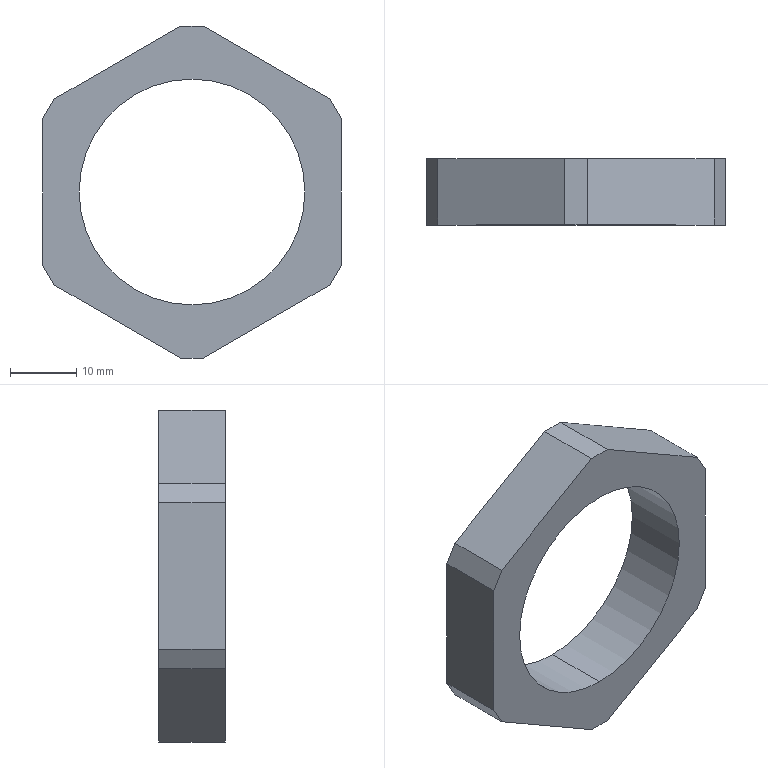Part | SolidWorks | features CirPattern 1, Extrusion 1, HoleWzd 1, ICE 1 | 1 solid | 16 faces | box 45 x 10 x 50 mm | volume 8358 mm3 | plane 14 | cylinder 2 | commonest cylinder face diameters 34 x2
STEP:
#1=CARTESIAN_POINT('',(0.,0.,-17.));
#2=VERTEX_POINT('',#1);
#3=CARTESIAN_POINT('',(0.,0.,17.));
#4=VERTEX_POINT('',#3);
#5=CARTESIAN_POINT('',(0.,0.,0.));
#6=DIRECTION('',(0.,1.,0.));
#7=DIRECTION('',(0.,0.,1.));
#8=AXIS2_PLACEMENT_3D('',#5,#6,#7);
#9=CIRCLE('',#8,17.);
#10=EDGE_CURVE('',#2,#4,#9,.T.);
#11=ORIENTED_EDGE('',*,*,#10,.F.);
#12=CARTESIAN_POINT('',(0.,10.,-17.));
#13=VERTEX_POINT('',#12);
#14=CARTESIAN_POINT('',(0.,10.,-17.));
#15=DIRECTION('',(0.,1.,0.));
#16=VECTOR('',#15,1000.);
#17=LINE('',#14,#16);
#18=EDGE_CURVE('',#2,#13,#17,.T.);
#19=ORIENTED_EDGE('',*,*,#18,.T.);
#20=CARTESIAN_POINT('',(0.,10.,17.));
#21=VERTEX_POINT('',#20);
#22=CARTESIAN_POINT('',(0.,10.,0.));
#23=DIRECTION('',(0.,1.,0.));
#24=DIRECTION('',(0.,0.,1.));
#25=AXIS2_PLACEMENT_3D('',#22,#23,#24);
#26=CIRCLE('',#25,17.);
#27=EDGE_CURVE('',#13,#21,#26,.T.);
#28=ORIENTED_EDGE('',*,*,#27,.T.);
#29=CARTESIAN_POINT('',(0.,10.,17.));
#30=DIRECTION('',(0.,1.,0.));
#31=VECTOR('',#30,1000.);
#32=LINE('',#29,#31);
#33=EDGE_CURVE('',#4,#21,#32,.T.);
#34=ORIENTED_EDGE('',*,*,#33,.F.);
#35=EDGE_LOOP('',(#11,#19,#28,#34));
#36=FACE_OUTER_BOUND('',#35,.T.);
#37=CARTESIAN_POINT('',(0.,10.,0.));
#38=DIRECTION('',(0.,1.,0.));
#39=DIRECTION('',(0.,0.,1.));
#40=AXIS2_PLACEMENT_3D('',#37,#38,#39);
#41=CYLINDRICAL_SURFACE('',#40,17.);
#42=ADVANCED_FACE('',(#36),#41,.F.);
#43=CARTESIAN_POINT('',(1.699,0.,25.));
#44=VERTEX_POINT('',#43);
#45=CARTESIAN_POINT('',(20.801,0.,13.971));
#46=VERTEX_POINT('',#45);
#47=CARTESIAN_POINT('',(0.,0.,25.981));
#48=DIRECTION('',(0.866,0.,-0.5));
#49=VECTOR('',#48,1000.);
#50=LINE('',#47,#49);
#51=EDGE_CURVE('',#44,#46,#50,.T.);
#52=ORIENTED_EDGE('',*,*,#51,.T.);
#53=CARTESIAN_POINT('',(20.801,10.,13.971));
#54=VERTEX_POINT('',#53);
#55=CARTESIAN_POINT('',(20.801,10.,13.971));
#56=DIRECTION('',(0.,1.,0.));
#57=VECTOR('',#56,1000.);
#58=LINE('',#55,#57);
#59=EDGE_CURVE('',#46,#54,#58,.T.);
#60=ORIENTED_EDGE('',*,*,#59,.T.);
#61=CARTESIAN_POINT('',(1.699,10.,25.));
#62=VERTEX_POINT('',#61);
#63=CARTESIAN_POINT('',(0.,10.,25.981));
#64=DIRECTION('',(0.866,0.,-0.5));
#65=VECTOR('',#64,1000.);
#66=LINE('',#63,#65);
#67=EDGE_CURVE('',#62,#54,#66,.T.);
#68=ORIENTED_EDGE('',*,*,#67,.F.);
#69=CARTESIAN_POINT('',(1.699,10.,25.));
#70=DIRECTION('',(0.,-1.,0.));
#71=VECTOR('',#70,1000.);
#72=LINE('',#69,#71);
#73=EDGE_CURVE('',#62,#44,#72,.T.);
#74=ORIENTED_EDGE('',*,*,#73,.T.);
#75=EDGE_LOOP('',(#52,#60,#68,#74));
#76=FACE_OUTER_BOUND('',#75,.T.);
#77=CARTESIAN_POINT('',(0.,10.,25.981));
#78=DIRECTION('',(-0.5,0.,-0.866));
#79=DIRECTION('',(-0.866,0.,0.5));
#80=AXIS2_PLACEMENT_3D('',#77,#78,#79);
#81=PLANE('',#80);
#82=ADVANCED_FACE('',(#76),#81,.F.);
#83=CARTESIAN_POINT('',(22.5,0.,11.029));
#84=VERTEX_POINT('',#83);
#85=CARTESIAN_POINT('',(22.5,0.,-11.029));
#86=VERTEX_POINT('',#85);
#87=CARTESIAN_POINT('',(22.5,0.,12.99));
#88=DIRECTION('',(0.,0.,-1.));
#89=VECTOR('',#88,1000.);
#90=LINE('',#87,#89);
#91=EDGE_CURVE('',#84,#86,#90,.T.);
#92=ORIENTED_EDGE('',*,*,#91,.T.);
#93=CARTESIAN_POINT('',(22.5,10.,-11.029));
#94=VERTEX_POINT('',#93);
#95=CARTESIAN_POINT('',(22.5,10.,-11.029));
#96=DIRECTION('',(0.,1.,0.));
#97=VECTOR('',#96,1000.);
#98=LINE('',#95,#97);
#99=EDGE_CURVE('',#86,#94,#98,.T.);
#100=ORIENTED_EDGE('',*,*,#99,.T.);
#101=CARTESIAN_POINT('',(22.5,10.,11.029));
#102=VERTEX_POINT('',#101);
#103=CARTESIAN_POINT('',(22.5,10.,12.99));
#104=DIRECTION('',(0.,0.,-1.));
#105=VECTOR('',#104,1000.);
#106=LINE('',#103,#105);
#107=EDGE_CURVE('',#102,#94,#106,.T.);
#108=ORIENTED_EDGE('',*,*,#107,.F.);
#109=CARTESIAN_POINT('',(22.5,10.,11.029));
#110=DIRECTION('',(0.,-1.,0.));
#111=VECTOR('',#110,1000.);
#112=LINE('',#109,#111);
#113=EDGE_CURVE('',#102,#84,#112,.T.);
#114=ORIENTED_EDGE('',*,*,#113,.T.);
#115=EDGE_LOOP('',(#92,#100,#108,#114));
#116=FACE_OUTER_BOUND('',#115,.T.);
#117=CARTESIAN_POINT('',(22.5,10.,12.99));
#118=DIRECTION('',(-1.,0.,0.));
#119=DIRECTION('',(0.,0.,1.));
#120=AXIS2_PLACEMENT_3D('',#117,#118,#119);
#121=PLANE('',#120);
#122=ADVANCED_FACE('',(#116),#121,.F.);
#123=CARTESIAN_POINT('',(20.801,10.,-13.971));
#124=VERTEX_POINT('',#123);
#125=CARTESIAN_POINT('',(1.699,10.,-25.));
#126=VERTEX_POINT('',#125);
#127=CARTESIAN_POINT('',(22.5,10.,-12.99));
#128=DIRECTION('',(-0.866,0.,-0.5));
#129=VECTOR('',#128,1000.);
#130=LINE('',#127,#129);
#131=EDGE_CURVE('',#124,#126,#130,.T.);
#132=ORIENTED_EDGE('',*,*,#131,.F.);
#133=CARTESIAN_POINT('',(20.801,0.,-13.971));
#134=VERTEX_POINT('',#133);
#135=CARTESIAN_POINT('',(20.801,10.,-13.971));
#136=DIRECTION('',(0.,-1.,0.));
#137=VECTOR('',#136,1000.);
#138=LINE('',#135,#137);
#139=EDGE_CURVE('',#124,#134,#138,.T.);
#140=ORIENTED_EDGE('',*,*,#139,.T.);
#141=CARTESIAN_POINT('',(1.699,0.,-25.));
#142=VERTEX_POINT('',#141);
#143=CARTESIAN_POINT('',(22.5,0.,-12.99));
#144=DIRECTION('',(-0.866,0.,-0.5));
#145=VECTOR('',#144,1000.);
#146=LINE('',#143,#145);
#147=EDGE_CURVE('',#134,#142,#146,.T.);
#148=ORIENTED_EDGE('',*,*,#147,.T.);
#149=CARTESIAN_POINT('',(1.699,10.,-25.));
#150=DIRECTION('',(0.,1.,0.));
#151=VECTOR('',#150,1000.);
#152=LINE('',#149,#151);
#153=EDGE_CURVE('',#142,#126,#152,.T.);
#154=ORIENTED_EDGE('',*,*,#153,.T.);
#155=EDGE_LOOP('',(#132,#140,#148,#154));
#156=FACE_OUTER_BOUND('',#155,.T.);
#157=CARTESIAN_POINT('',(22.5,10.,-12.99));
#158=DIRECTION('',(-0.5,0.,0.866));
#159=DIRECTION('',(0.866,0.,0.5));
#160=AXIS2_PLACEMENT_3D('',#157,#158,#159);
#161=PLANE('',#160);
#162=ADVANCED_FACE('',(#156),#161,.F.);
#163=CARTESIAN_POINT('',(-1.699,0.,-25.));
#164=VERTEX_POINT('',#163);
#165=CARTESIAN_POINT('',(-20.801,0.,-13.971));
#166=VERTEX_POINT('',#165);
#167=CARTESIAN_POINT('',(0.,0.,-25.981));
#168=DIRECTION('',(-0.866,0.,0.5));
#169=VECTOR('',#168,1000.);
#170=LINE('',#167,#169);
#171=EDGE_CURVE('',#164,#166,#170,.T.);
#172=ORIENTED_EDGE('',*,*,#171,.T.);
#173=CARTESIAN_POINT('',(-20.801,10.,-13.971));
#174=VERTEX_POINT('',#173);
#175=CARTESIAN_POINT('',(-20.801,10.,-13.971));
#176=DIRECTION('',(0.,1.,0.));
#177=VECTOR('',#176,1000.);
#178=LINE('',#175,#177);
#179=EDGE_CURVE('',#166,#174,#178,.T.);
#180=ORIENTED_EDGE('',*,*,#179,.T.);
#181=CARTESIAN_POINT('',(-1.699,10.,-25.));
#182=VERTEX_POINT('',#181);
#183=CARTESIAN_POINT('',(0.,10.,-25.981));
#184=DIRECTION('',(-0.866,0.,0.5));
#185=VECTOR('',#184,1000.);
#186=LINE('',#183,#185);
#187=EDGE_CURVE('',#182,#174,#186,.T.);
#188=ORIENTED_EDGE('',*,*,#187,.F.);
#189=CARTESIAN_POINT('',(-1.699,10.,-25.));
#190=DIRECTION('',(0.,-1.,0.));
#191=VECTOR('',#190,1000.);
#192=LINE('',#189,#191);
#193=EDGE_CURVE('',#182,#164,#192,.T.);
#194=ORIENTED_EDGE('',*,*,#193,.T.);
#195=EDGE_LOOP('',(#172,#180,#188,#194));
#196=FACE_OUTER_BOUND('',#195,.T.);
#197=CARTESIAN_POINT('',(0.,10.,-25.981));
#198=DIRECTION('',(0.5,0.,0.866));
#199=DIRECTION('',(0.866,0.,-0.5));
#200=AXIS2_PLACEMENT_3D('',#197,#198,#199);
#201=PLANE('',#200);
#202=ADVANCED_FACE('',(#196),#201,.F.);
#203=CARTESIAN_POINT('',(-22.5,0.,-11.029));
#204=VERTEX_POINT('',#203);
#205=CARTESIAN_POINT('',(-22.5,0.,11.029));
#206=VERTEX_POINT('',#205);
#207=CARTESIAN_POINT('',(-22.5,0.,-12.99));
#208=DIRECTION('',(0.,0.,1.));
#209=VECTOR('',#208,1000.);
#210=LINE('',#207,#209);
#211=EDGE_CURVE('',#204,#206,#210,.T.);
#212=ORIENTED_EDGE('',*,*,#211,.T.);
#213=CARTESIAN_POINT('',(-22.5,10.,11.029));
#214=VERTEX_POINT('',#213);
#215=CARTESIAN_POINT('',(-22.5,10.,11.029));
#216=DIRECTION('',(0.,1.,0.));
#217=VECTOR('',#216,1000.);
#218=LINE('',#215,#217);
#219=EDGE_CURVE('',#206,#214,#218,.T.);
#220=ORIENTED_EDGE('',*,*,#219,.T.);
#221=CARTESIAN_POINT('',(-22.5,10.,-11.029));
#222=VERTEX_POINT('',#221);
#223=CARTESIAN_POINT('',(-22.5,10.,-12.99));
#224=DIRECTION('',(0.,0.,1.));
#225=VECTOR('',#224,1000.);
#226=LINE('',#223,#225);
#227=EDGE_CURVE('',#222,#214,#226,.T.);
#228=ORIENTED_EDGE('',*,*,#227,.F.);
#229=CARTESIAN_POINT('',(-22.5,10.,-11.029));
#230=DIRECTION('',(0.,-1.,0.));
#231=VECTOR('',#230,1000.);
#232=LINE('',#229,#231);
#233=EDGE_CURVE('',#222,#204,#232,.T.);
#234=ORIENTED_EDGE('',*,*,#233,.T.);
#235=EDGE_LOOP('',(#212,#220,#228,#234));
#236=FACE_OUTER_BOUND('',#235,.T.);
#237=CARTESIAN_POINT('',(-22.5,10.,-12.99));
#238=DIRECTION('',(1.,0.,0.));
#239=DIRECTION('',(0.,0.,-1.));
#240=AXIS2_PLACEMENT_3D('',#237,#238,#239);
#241=PLANE('',#240);
#242=ADVANCED_FACE('',(#236),#241,.F.);
#243=CARTESIAN_POINT('',(-20.801,0.,13.971));
#244=VERTEX_POINT('',#243);
#245=CARTESIAN_POINT('',(-1.699,0.,25.));
#246=VERTEX_POINT('',#245);
#247=CARTESIAN_POINT('',(-22.5,0.,12.99));
#248=DIRECTION('',(0.866,0.,0.5));
#249=VECTOR('',#248,1000.);
#250=LINE('',#247,#249);
#251=EDGE_CURVE('',#244,#246,#250,.T.);
#252=ORIENTED_EDGE('',*,*,#251,.T.);
#253=CARTESIAN_POINT('',(-1.699,10.,25.));
#254=VERTEX_POINT('',#253);
#255=CARTESIAN_POINT('',(-1.699,10.,25.));
#256=DIRECTION('',(0.,1.,0.));
#257=VECTOR('',#256,1000.);
#258=LINE('',#255,#257);
#259=EDGE_CURVE('',#246,#254,#258,.T.);
#260=ORIENTED_EDGE('',*,*,#259,.T.);
#261=CARTESIAN_POINT('',(-20.801,10.,13.971));
#262=VERTEX_POINT('',#261);
#263=CARTESIAN_POINT('',(-22.5,10.,12.99));
#264=DIRECTION('',(0.866,0.,0.5));
#265=VECTOR('',#264,1000.);
#266=LINE('',#263,#265);
#267=EDGE_CURVE('',#262,#254,#266,.T.);
#268=ORIENTED_EDGE('',*,*,#267,.F.);
#269=CARTESIAN_POINT('',(-20.801,10.,13.971));
#270=DIRECTION('',(0.,-1.,0.));
#271=VECTOR('',#270,1000.);
#272=LINE('',#269,#271);
#273=EDGE_CURVE('',#262,#244,#272,.T.);
#274=ORIENTED_EDGE('',*,*,#273,.T.);
#275=EDGE_LOOP('',(#252,#260,#268,#274));
#276=FACE_OUTER_BOUND('',#275,.T.);
#277=CARTESIAN_POINT('',(-22.5,10.,12.99));
#278=DIRECTION('',(0.5,0.,-0.866));
#279=DIRECTION('',(-0.866,0.,-0.5));
#280=AXIS2_PLACEMENT_3D('',#277,#278,#279);
#281=PLANE('',#280);
#282=ADVANCED_FACE('',(#276),#281,.F.);
#283=CARTESIAN_POINT('',(17.53,10.,-19.637));
#284=DIRECTION('',(0.5,0.,0.866));
#285=VECTOR('',#284,1000.);
#286=LINE('',#283,#285);
#287=EDGE_CURVE('',#124,#94,#286,.T.);
#288=ORIENTED_EDGE('',*,*,#287,.F.);
#289=ORIENTED_EDGE('',*,*,#131,.T.);
#290=CARTESIAN_POINT('',(-8.241,10.,-25.));
#291=DIRECTION('',(1.,0.,0.));
#292=VECTOR('',#291,1000.);
#293=LINE('',#290,#292);
#294=EDGE_CURVE('',#182,#126,#293,.T.);
#295=ORIENTED_EDGE('',*,*,#294,.F.);
#296=ORIENTED_EDGE('',*,*,#187,.T.);
#297=CARTESIAN_POINT('',(-25.771,10.,-5.363));
#298=DIRECTION('',(0.5,0.,-0.866));
#299=VECTOR('',#298,1000.);
#300=LINE('',#297,#299);
#301=EDGE_CURVE('',#222,#174,#300,.T.);
#302=ORIENTED_EDGE('',*,*,#301,.F.);
#303=ORIENTED_EDGE('',*,*,#227,.T.);
#304=CARTESIAN_POINT('',(-17.53,10.,19.637));
#305=DIRECTION('',(-0.5,0.,-0.866));
#306=VECTOR('',#305,1000.);
#307=LINE('',#304,#306);
#308=EDGE_CURVE('',#262,#214,#307,.T.);
#309=ORIENTED_EDGE('',*,*,#308,.F.);
#310=ORIENTED_EDGE('',*,*,#267,.T.);
#311=CARTESIAN_POINT('',(8.241,10.,25.));
#312=DIRECTION('',(-1.,0.,0.));
#313=VECTOR('',#312,1000.);
#314=LINE('',#311,#313);
#315=EDGE_CURVE('',#62,#254,#314,.T.);
#316=ORIENTED_EDGE('',*,*,#315,.F.);
#317=ORIENTED_EDGE('',*,*,#67,.T.);
#318=CARTESIAN_POINT('',(25.771,10.,5.363));
#319=DIRECTION('',(-0.5,0.,0.866));
#320=VECTOR('',#319,1000.);
#321=LINE('',#318,#320);
#322=EDGE_CURVE('',#102,#54,#321,.T.);
#323=ORIENTED_EDGE('',*,*,#322,.F.);
#324=ORIENTED_EDGE('',*,*,#107,.T.);
#325=EDGE_LOOP('',(#288,#289,#295,#296,#302,#303,#309,#310,#316,#317,#323,#324));
#326=FACE_OUTER_BOUND('',#325,.T.);
#327=CARTESIAN_POINT('',(0.,10.,0.));
#328=DIRECTION('',(0.,1.,0.));
#329=DIRECTION('',(0.,0.,1.));
#330=AXIS2_PLACEMENT_3D('',#327,#328,#329);
#331=CIRCLE('',#330,17.);
#332=EDGE_CURVE('',#21,#13,#331,.T.);
#333=ORIENTED_EDGE('',*,*,#332,.F.);
#334=ORIENTED_EDGE('',*,*,#27,.F.);
#335=EDGE_LOOP('',(#333,#334));
#336=FACE_BOUND('',#335,.T.);
#337=CARTESIAN_POINT('',(0.,10.,0.));
#338=DIRECTION('',(0.,1.,0.));
#339=DIRECTION('',(0.,0.,1.));
#340=AXIS2_PLACEMENT_3D('',#337,#338,#339);
#341=PLANE('',#340);
#342=ADVANCED_FACE('',(#326,#336),#341,.T.);
#343=CARTESIAN_POINT('',(0.,0.,0.));
#344=DIRECTION('',(0.,1.,0.));
#345=DIRECTION('',(0.,0.,1.));
#346=AXIS2_PLACEMENT_3D('',#343,#344,#345);
#347=CIRCLE('',#346,17.);
#348=EDGE_CURVE('',#4,#2,#347,.T.);
#349=ORIENTED_EDGE('',*,*,#348,.T.);
#350=ORIENTED_EDGE('',*,*,#10,.T.);
#351=EDGE_LOOP('',(#349,#350));
#352=FACE_BOUND('',#351,.T.);
#353=ORIENTED_EDGE('',*,*,#147,.F.);
#354=CARTESIAN_POINT('',(21.651,0.,-12.5));
#355=DIRECTION('',(0.5,0.,0.866));
#356=VECTOR('',#355,1000.);
#357=LINE('',#354,#356);
#358=EDGE_CURVE('',#134,#86,#357,.T.);
#359=ORIENTED_EDGE('',*,*,#358,.T.);
#360=ORIENTED_EDGE('',*,*,#91,.F.);
#361=CARTESIAN_POINT('',(21.651,0.,12.5));
#362=DIRECTION('',(-0.5,0.,0.866));
#363=VECTOR('',#362,1000.);
#364=LINE('',#361,#363);
#365=EDGE_CURVE('',#84,#46,#364,.T.);
#366=ORIENTED_EDGE('',*,*,#365,.T.);
#367=ORIENTED_EDGE('',*,*,#51,.F.);
#368=CARTESIAN_POINT('',(0.,0.,25.));
#369=DIRECTION('',(-1.,0.,0.));
#370=VECTOR('',#369,1000.);
#371=LINE('',#368,#370);
#372=EDGE_CURVE('',#44,#246,#371,.T.);
#373=ORIENTED_EDGE('',*,*,#372,.T.);
#374=ORIENTED_EDGE('',*,*,#251,.F.);
#375=CARTESIAN_POINT('',(-21.651,0.,12.5));
#376=DIRECTION('',(-0.5,0.,-0.866));
#377=VECTOR('',#376,1000.);
#378=LINE('',#375,#377);
#379=EDGE_CURVE('',#244,#206,#378,.T.);
#380=ORIENTED_EDGE('',*,*,#379,.T.);
#381=ORIENTED_EDGE('',*,*,#211,.F.);
#382=CARTESIAN_POINT('',(-21.651,0.,-12.5));
#383=DIRECTION('',(0.5,0.,-0.866));
#384=VECTOR('',#383,1000.);
#385=LINE('',#382,#384);
#386=EDGE_CURVE('',#204,#166,#385,.T.);
#387=ORIENTED_EDGE('',*,*,#386,.T.);
#388=ORIENTED_EDGE('',*,*,#171,.F.);
#389=CARTESIAN_POINT('',(0.,0.,-25.));
#390=DIRECTION('',(1.,0.,0.));
#391=VECTOR('',#390,1000.);
#392=LINE('',#389,#391);
#393=EDGE_CURVE('',#164,#142,#392,.T.);
#394=ORIENTED_EDGE('',*,*,#393,.T.);
#395=EDGE_LOOP('',(#353,#359,#360,#366,#367,#373,#374,#380,#381,#387,#388,#394));
#396=FACE_OUTER_BOUND('',#395,.T.);
#397=CARTESIAN_POINT('',(0.,0.,0.));
#398=DIRECTION('',(0.,1.,0.));
#399=DIRECTION('',(0.,0.,1.));
#400=AXIS2_PLACEMENT_3D('',#397,#398,#399);
#401=PLANE('',#400);
#402=ADVANCED_FACE('',(#352,#396),#401,.F.);
#403=ORIENTED_EDGE('',*,*,#18,.F.);
#404=ORIENTED_EDGE('',*,*,#348,.F.);
#405=ORIENTED_EDGE('',*,*,#33,.T.);
#406=ORIENTED_EDGE('',*,*,#332,.T.);
#407=EDGE_LOOP('',(#403,#404,#405,#406));
#408=FACE_OUTER_BOUND('',#407,.T.);
#409=CARTESIAN_POINT('',(0.,10.,0.));
#410=DIRECTION('',(0.,1.,0.));
#411=DIRECTION('',(0.,0.,1.));
#412=AXIS2_PLACEMENT_3D('',#409,#410,#411);
#413=CYLINDRICAL_SURFACE('',#412,17.);
#414=ADVANCED_FACE('',(#408),#413,.F.);
#415=ORIENTED_EDGE('',*,*,#393,.F.);
#416=ORIENTED_EDGE('',*,*,#193,.F.);
#417=ORIENTED_EDGE('',*,*,#294,.T.);
#418=ORIENTED_EDGE('',*,*,#153,.F.);
#419=EDGE_LOOP('',(#415,#416,#417,#418));
#420=FACE_OUTER_BOUND('',#419,.T.);
#421=CARTESIAN_POINT('',(-8.241,-78.,-25.));
#422=DIRECTION('',(0.,0.,1.));
#423=DIRECTION('',(1.,0.,0.));
#424=AXIS2_PLACEMENT_3D('',#421,#422,#423);
#425=PLANE('',#424);
#426=ADVANCED_FACE('',(#420),#425,.F.);
#427=ORIENTED_EDGE('',*,*,#386,.F.);
#428=ORIENTED_EDGE('',*,*,#233,.F.);
#429=ORIENTED_EDGE('',*,*,#301,.T.);
#430=ORIENTED_EDGE('',*,*,#179,.F.);
#431=EDGE_LOOP('',(#427,#428,#429,#430));
#432=FACE_OUTER_BOUND('',#431,.T.);
#433=CARTESIAN_POINT('',(-25.771,-78.,-5.363));
#434=DIRECTION('',(0.866,0.,0.5));
#435=DIRECTION('',(0.5,0.,-0.866));
#436=AXIS2_PLACEMENT_3D('',#433,#434,#435);
#437=PLANE('',#436);
#438=ADVANCED_FACE('',(#432),#437,.F.);
#439=ORIENTED_EDGE('',*,*,#379,.F.);
#440=ORIENTED_EDGE('',*,*,#273,.F.);
#441=ORIENTED_EDGE('',*,*,#308,.T.);
#442=ORIENTED_EDGE('',*,*,#219,.F.);
#443=EDGE_LOOP('',(#439,#440,#441,#442));
#444=FACE_OUTER_BOUND('',#443,.T.);
#445=CARTESIAN_POINT('',(-17.53,-78.,19.637));
#446=DIRECTION('',(0.866,0.,-0.5));
#447=DIRECTION('',(-0.5,0.,-0.866));
#448=AXIS2_PLACEMENT_3D('',#445,#446,#447);
#449=PLANE('',#448);
#450=ADVANCED_FACE('',(#444),#449,.F.);
#451=ORIENTED_EDGE('',*,*,#315,.T.);
#452=ORIENTED_EDGE('',*,*,#259,.F.);
#453=ORIENTED_EDGE('',*,*,#372,.F.);
#454=ORIENTED_EDGE('',*,*,#73,.F.);
#455=EDGE_LOOP('',(#451,#452,#453,#454));
#456=FACE_OUTER_BOUND('',#455,.T.);
#457=CARTESIAN_POINT('',(8.241,-78.,25.));
#458=DIRECTION('',(0.,0.,-1.));
#459=DIRECTION('',(-1.,0.,0.));
#460=AXIS2_PLACEMENT_3D('',#457,#458,#459);
#461=PLANE('',#460);
#462=ADVANCED_FACE('',(#456),#461,.F.);
#463=ORIENTED_EDGE('',*,*,#365,.F.);
#464=ORIENTED_EDGE('',*,*,#113,.F.);
#465=ORIENTED_EDGE('',*,*,#322,.T.);
#466=ORIENTED_EDGE('',*,*,#59,.F.);
#467=EDGE_LOOP('',(#463,#464,#465,#466));
#468=FACE_OUTER_BOUND('',#467,.T.);
#469=CARTESIAN_POINT('',(25.771,-78.,5.363));
#470=DIRECTION('',(-0.866,0.,-0.5));
#471=DIRECTION('',(-0.5,0.,0.866));
#472=AXIS2_PLACEMENT_3D('',#469,#470,#471);
#473=PLANE('',#472);
#474=ADVANCED_FACE('',(#468),#473,.F.);
#475=ORIENTED_EDGE('',*,*,#358,.F.);
#476=ORIENTED_EDGE('',*,*,#139,.F.);
#477=ORIENTED_EDGE('',*,*,#287,.T.);
#478=ORIENTED_EDGE('',*,*,#99,.F.);
#479=EDGE_LOOP('',(#475,#476,#477,#478));
#480=FACE_OUTER_BOUND('',#479,.T.);
#481=CARTESIAN_POINT('',(17.53,-78.,-19.637));
#482=DIRECTION('',(-0.866,0.,0.5));
#483=DIRECTION('',(0.5,0.,0.866));
#484=AXIS2_PLACEMENT_3D('',#481,#482,#483);
#485=PLANE('',#484);
#486=ADVANCED_FACE('',(#480),#485,.F.);
#487=CLOSED_SHELL('',(#42,#82,#122,#162,#202,#242,#282,#342,#402,#414,#426,#438,#450,#462,#474,#486));
#488=MANIFOLD_SOLID_BREP('',#487);
#489=CARTESIAN_POINT('',(0.,0.,0.));
#490=DIRECTION('',(0.,0.,1.));
#491=DIRECTION('',(1.,0.,0.));
#492=AXIS2_PLACEMENT_3D('',#489,#490,#491);
#493=(LENGTH_UNIT()NAMED_UNIT(*)SI_UNIT(.MILLI.,.METRE.));
#494=UNCERTAINTY_MEASURE_WITH_UNIT(LENGTH_MEASURE(0.00001),#493,'','');
#495=(NAMED_UNIT(*)PLANE_ANGLE_UNIT()SI_UNIT($,.RADIAN.));
#496=(NAMED_UNIT(*)SI_UNIT($,.STERADIAN.)SOLID_ANGLE_UNIT());
#497=(GEOMETRIC_REPRESENTATION_CONTEXT(3)GLOBAL_UNCERTAINTY_ASSIGNED_CONTEXT((#494))GLOBAL_UNIT_ASSIGNED_CONTEXT((#493,#495,#496))REPRESENTATION_CONTEXT('',''));
#498=ADVANCED_BREP_SHAPE_REPRESENTATION('',(#488,#492),#497);